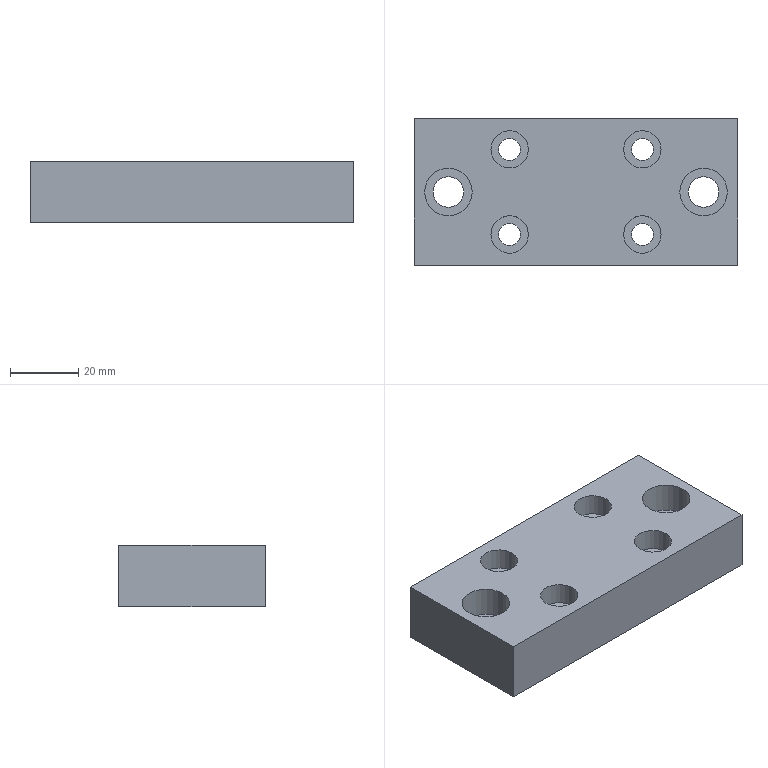Part | STEP file | lll_id474_x_t | 1 solid | 24 faces | box 95 x 43 x 18 mm | volume 65617 mm3 | plane 12 | cylinder 12 | commonest cylinder face diameters 6.5 x4 11 x4 9 x2 14 x2
STEP:
#1=CARTESIAN_POINT('',(47.5,65.,137.5));
#2=VERTEX_POINT('',#1);
#3=CARTESIAN_POINT('',(-47.5,65.,137.5));
#4=VERTEX_POINT('',#3);
#5=CARTESIAN_POINT('',(0.,65.,137.5));
#6=DIRECTION('',(-1.,0.,0.));
#7=VECTOR('',#6,1.);
#8=LINE('',#5,#7);
#9=EDGE_CURVE('',#2,#4,#8,.T.);
#10=ORIENTED_EDGE('',*,*,#9,.F.);
#11=CARTESIAN_POINT('',(47.5,65.,155.5));
#12=VERTEX_POINT('',#11);
#13=CARTESIAN_POINT('',(47.5,65.,155.5));
#14=DIRECTION('',(0.,0.,-1.));
#15=VECTOR('',#14,1.);
#16=LINE('',#13,#15);
#17=EDGE_CURVE('',#12,#2,#16,.T.);
#18=ORIENTED_EDGE('',*,*,#17,.F.);
#19=CARTESIAN_POINT('',(-47.5,65.,155.5));
#20=VERTEX_POINT('',#19);
#21=CARTESIAN_POINT('',(0.,65.,155.5));
#22=DIRECTION('',(-1.,0.,0.));
#23=VECTOR('',#22,1.);
#24=LINE('',#21,#23);
#25=EDGE_CURVE('',#12,#20,#24,.T.);
#26=ORIENTED_EDGE('',*,*,#25,.T.);
#27=CARTESIAN_POINT('',(-47.5,65.,155.5));
#28=DIRECTION('',(0.,0.,-1.));
#29=VECTOR('',#28,1.);
#30=LINE('',#27,#29);
#31=EDGE_CURVE('',#20,#4,#30,.T.);
#32=ORIENTED_EDGE('',*,*,#31,.T.);
#33=EDGE_LOOP('',(#10,#18,#26,#32));
#34=FACE_OUTER_BOUND('',#33,.T.);
#35=CARTESIAN_POINT('',(0.,65.,155.5));
#36=DIRECTION('',(0.,-1.,0.));
#37=DIRECTION('',(0.,0.,-1.));
#38=AXIS2_PLACEMENT_3D('',#35,#36,#37);
#39=PLANE('',#38);
#40=ADVANCED_FACE('',(#34),#39,.T.);
#41=CARTESIAN_POINT('',(47.5,108.,137.5));
#42=VERTEX_POINT('',#41);
#43=CARTESIAN_POINT('',(47.5,140.161,137.5));
#44=DIRECTION('',(0.,-1.,0.));
#45=VECTOR('',#44,1.);
#46=LINE('',#43,#45);
#47=EDGE_CURVE('',#42,#2,#46,.T.);
#48=ORIENTED_EDGE('',*,*,#47,.F.);
#49=CARTESIAN_POINT('',(47.5,108.,155.5));
#50=VERTEX_POINT('',#49);
#51=CARTESIAN_POINT('',(47.5,108.,155.5));
#52=DIRECTION('',(0.,0.,-1.));
#53=VECTOR('',#52,1.);
#54=LINE('',#51,#53);
#55=EDGE_CURVE('',#50,#42,#54,.T.);
#56=ORIENTED_EDGE('',*,*,#55,.F.);
#57=CARTESIAN_POINT('',(47.5,140.161,155.5));
#58=DIRECTION('',(0.,-1.,0.));
#59=VECTOR('',#58,1.);
#60=LINE('',#57,#59);
#61=EDGE_CURVE('',#50,#12,#60,.T.);
#62=ORIENTED_EDGE('',*,*,#61,.T.);
#63=ORIENTED_EDGE('',*,*,#17,.T.);
#64=EDGE_LOOP('',(#48,#56,#62,#63));
#65=FACE_OUTER_BOUND('',#64,.T.);
#66=CARTESIAN_POINT('',(47.5,140.161,155.5));
#67=DIRECTION('',(1.,0.,0.));
#68=DIRECTION('',(0.,0.,-1.));
#69=AXIS2_PLACEMENT_3D('',#66,#67,#68);
#70=PLANE('',#69);
#71=ADVANCED_FACE('',(#65),#70,.T.);
#72=CARTESIAN_POINT('',(-47.5,108.,137.5));
#73=VERTEX_POINT('',#72);
#74=CARTESIAN_POINT('',(0.,108.,137.5));
#75=DIRECTION('',(-1.,0.,0.));
#76=VECTOR('',#75,1.);
#77=LINE('',#74,#76);
#78=EDGE_CURVE('',#42,#73,#77,.T.);
#79=ORIENTED_EDGE('',*,*,#78,.T.);
#80=CARTESIAN_POINT('',(-47.5,108.,155.5));
#81=VERTEX_POINT('',#80);
#82=CARTESIAN_POINT('',(-47.5,108.,155.5));
#83=DIRECTION('',(0.,0.,-1.));
#84=VECTOR('',#83,1.);
#85=LINE('',#82,#84);
#86=EDGE_CURVE('',#81,#73,#85,.T.);
#87=ORIENTED_EDGE('',*,*,#86,.F.);
#88=CARTESIAN_POINT('',(0.,108.,155.5));
#89=DIRECTION('',(-1.,0.,0.));
#90=VECTOR('',#89,1.);
#91=LINE('',#88,#90);
#92=EDGE_CURVE('',#50,#81,#91,.T.);
#93=ORIENTED_EDGE('',*,*,#92,.F.);
#94=ORIENTED_EDGE('',*,*,#55,.T.);
#95=EDGE_LOOP('',(#79,#87,#93,#94));
#96=FACE_OUTER_BOUND('',#95,.T.);
#97=CARTESIAN_POINT('',(0.,108.,155.5));
#98=DIRECTION('',(0.,-1.,0.));
#99=DIRECTION('',(0.,0.,-1.));
#100=AXIS2_PLACEMENT_3D('',#97,#98,#99);
#101=PLANE('',#100);
#102=ADVANCED_FACE('',(#96),#101,.F.);
#103=CARTESIAN_POINT('',(-47.5,0.,137.5));
#104=DIRECTION('',(0.,-1.,0.));
#105=VECTOR('',#104,1.);
#106=LINE('',#103,#105);
#107=EDGE_CURVE('',#73,#4,#106,.T.);
#108=ORIENTED_EDGE('',*,*,#107,.T.);
#109=ORIENTED_EDGE('',*,*,#31,.F.);
#110=CARTESIAN_POINT('',(-47.5,0.,155.5));
#111=DIRECTION('',(0.,-1.,0.));
#112=VECTOR('',#111,1.);
#113=LINE('',#110,#112);
#114=EDGE_CURVE('',#81,#20,#113,.T.);
#115=ORIENTED_EDGE('',*,*,#114,.F.);
#116=ORIENTED_EDGE('',*,*,#86,.T.);
#117=EDGE_LOOP('',(#108,#109,#115,#116));
#118=FACE_OUTER_BOUND('',#117,.T.);
#119=CARTESIAN_POINT('',(-47.5,0.,155.5));
#120=DIRECTION('',(1.,0.,0.));
#121=DIRECTION('',(0.,0.,-1.));
#122=AXIS2_PLACEMENT_3D('',#119,#120,#121);
#123=PLANE('',#122);
#124=ADVANCED_FACE('',(#118),#123,.F.);
#125=CARTESIAN_POINT('',(25.,99.,155.5));
#126=VERTEX_POINT('',#125);
#127=CARTESIAN_POINT('',(19.5,99.,155.5));
#128=DIRECTION('',(0.,0.,-1.));
#129=DIRECTION('',(1.,0.,0.));
#130=AXIS2_PLACEMENT_3D('',#127,#128,#129);
#131=CIRCLE('',#130,5.5);
#132=EDGE_CURVE('',#126,#126,#131,.T.);
#133=ORIENTED_EDGE('',*,*,#132,.T.);
#134=EDGE_LOOP('',(#133));
#135=FACE_BOUND('',#134,.T.);
#136=CARTESIAN_POINT('',(-25.,99.,155.5));
#137=VERTEX_POINT('',#136);
#138=CARTESIAN_POINT('',(-19.5,99.,155.5));
#139=DIRECTION('',(0.,0.,1.));
#140=DIRECTION('',(-1.,0.,0.));
#141=AXIS2_PLACEMENT_3D('',#138,#139,#140);
#142=CIRCLE('',#141,5.5);
#143=EDGE_CURVE('',#137,#137,#142,.T.);
#144=ORIENTED_EDGE('',*,*,#143,.F.);
#145=EDGE_LOOP('',(#144));
#146=FACE_BOUND('',#145,.T.);
#147=CARTESIAN_POINT('',(25.,74.,155.5));
#148=VERTEX_POINT('',#147);
#149=CARTESIAN_POINT('',(19.5,74.,155.5));
#150=DIRECTION('',(0.,0.,1.));
#151=DIRECTION('',(1.,0.,0.));
#152=AXIS2_PLACEMENT_3D('',#149,#150,#151);
#153=CIRCLE('',#152,5.5);
#154=EDGE_CURVE('',#148,#148,#153,.T.);
#155=ORIENTED_EDGE('',*,*,#154,.F.);
#156=EDGE_LOOP('',(#155));
#157=FACE_BOUND('',#156,.T.);
#158=CARTESIAN_POINT('',(-25.,74.,155.5));
#159=VERTEX_POINT('',#158);
#160=CARTESIAN_POINT('',(-19.5,74.,155.5));
#161=DIRECTION('',(0.,0.,-1.));
#162=DIRECTION('',(-1.,0.,0.));
#163=AXIS2_PLACEMENT_3D('',#160,#161,#162);
#164=CIRCLE('',#163,5.5);
#165=EDGE_CURVE('',#159,#159,#164,.T.);
#166=ORIENTED_EDGE('',*,*,#165,.T.);
#167=EDGE_LOOP('',(#166));
#168=FACE_BOUND('',#167,.T.);
#169=CARTESIAN_POINT('',(-30.5,86.5,155.5));
#170=VERTEX_POINT('',#169);
#171=CARTESIAN_POINT('',(-37.5,86.5,155.5));
#172=DIRECTION('',(0.,0.,1.));
#173=DIRECTION('',(1.,0.,0.));
#174=AXIS2_PLACEMENT_3D('',#171,#172,#173);
#175=CIRCLE('',#174,7.);
#176=EDGE_CURVE('',#170,#170,#175,.T.);
#177=ORIENTED_EDGE('',*,*,#176,.F.);
#178=EDGE_LOOP('',(#177));
#179=FACE_BOUND('',#178,.T.);
#180=CARTESIAN_POINT('',(30.5,86.5,155.5));
#181=VERTEX_POINT('',#180);
#182=CARTESIAN_POINT('',(37.5,86.5,155.5));
#183=DIRECTION('',(0.,0.,-1.));
#184=DIRECTION('',(-1.,0.,0.));
#185=AXIS2_PLACEMENT_3D('',#182,#183,#184);
#186=CIRCLE('',#185,7.);
#187=EDGE_CURVE('',#181,#181,#186,.T.);
#188=ORIENTED_EDGE('',*,*,#187,.T.);
#189=EDGE_LOOP('',(#188));
#190=FACE_BOUND('',#189,.T.);
#191=ORIENTED_EDGE('',*,*,#25,.F.);
#192=ORIENTED_EDGE('',*,*,#61,.F.);
#193=ORIENTED_EDGE('',*,*,#92,.T.);
#194=ORIENTED_EDGE('',*,*,#114,.T.);
#195=EDGE_LOOP('',(#191,#192,#193,#194));
#196=FACE_BOUND('',#195,.T.);
#197=CARTESIAN_POINT('',(0.,0.,155.5));
#198=DIRECTION('',(0.,0.,1.));
#199=DIRECTION('',(1.,0.,0.));
#200=AXIS2_PLACEMENT_3D('',#197,#198,#199);
#201=PLANE('',#200);
#202=ADVANCED_FACE('',(#135,#146,#157,#168,#179,#190,#196),#201,.T.);
#203=CARTESIAN_POINT('',(22.75,99.,137.5));
#204=VERTEX_POINT('',#203);
#205=CARTESIAN_POINT('',(19.5,99.,137.5));
#206=DIRECTION('',(0.,0.,1.));
#207=DIRECTION('',(1.,0.,0.));
#208=AXIS2_PLACEMENT_3D('',#205,#206,#207);
#209=CIRCLE('',#208,3.25);
#210=EDGE_CURVE('',#204,#204,#209,.T.);
#211=ORIENTED_EDGE('',*,*,#210,.T.);
#212=EDGE_LOOP('',(#211));
#213=FACE_BOUND('',#212,.T.);
#214=CARTESIAN_POINT('',(-16.25,99.,137.5));
#215=VERTEX_POINT('',#214);
#216=CARTESIAN_POINT('',(-19.5,99.,137.5));
#217=DIRECTION('',(0.,0.,1.));
#218=DIRECTION('',(1.,0.,0.));
#219=AXIS2_PLACEMENT_3D('',#216,#217,#218);
#220=CIRCLE('',#219,3.25);
#221=EDGE_CURVE('',#215,#215,#220,.T.);
#222=ORIENTED_EDGE('',*,*,#221,.T.);
#223=EDGE_LOOP('',(#222));
#224=FACE_BOUND('',#223,.T.);
#225=CARTESIAN_POINT('',(22.75,74.,137.5));
#226=VERTEX_POINT('',#225);
#227=CARTESIAN_POINT('',(19.5,74.,137.5));
#228=DIRECTION('',(0.,0.,1.));
#229=DIRECTION('',(1.,0.,0.));
#230=AXIS2_PLACEMENT_3D('',#227,#228,#229);
#231=CIRCLE('',#230,3.25);
#232=EDGE_CURVE('',#226,#226,#231,.T.);
#233=ORIENTED_EDGE('',*,*,#232,.T.);
#234=EDGE_LOOP('',(#233));
#235=FACE_BOUND('',#234,.T.);
#236=CARTESIAN_POINT('',(-16.25,74.,137.5));
#237=VERTEX_POINT('',#236);
#238=CARTESIAN_POINT('',(-19.5,74.,137.5));
#239=DIRECTION('',(0.,0.,1.));
#240=DIRECTION('',(1.,0.,0.));
#241=AXIS2_PLACEMENT_3D('',#238,#239,#240);
#242=CIRCLE('',#241,3.25);
#243=EDGE_CURVE('',#237,#237,#242,.T.);
#244=ORIENTED_EDGE('',*,*,#243,.T.);
#245=EDGE_LOOP('',(#244));
#246=FACE_BOUND('',#245,.T.);
#247=CARTESIAN_POINT('',(-33.,86.5,137.5));
#248=VERTEX_POINT('',#247);
#249=CARTESIAN_POINT('',(-37.5,86.5,137.5));
#250=DIRECTION('',(0.,0.,1.));
#251=DIRECTION('',(1.,0.,0.));
#252=AXIS2_PLACEMENT_3D('',#249,#250,#251);
#253=CIRCLE('',#252,4.5);
#254=EDGE_CURVE('',#248,#248,#253,.T.);
#255=ORIENTED_EDGE('',*,*,#254,.T.);
#256=EDGE_LOOP('',(#255));
#257=FACE_BOUND('',#256,.T.);
#258=CARTESIAN_POINT('',(42.,86.5,137.5));
#259=VERTEX_POINT('',#258);
#260=CARTESIAN_POINT('',(37.5,86.5,137.5));
#261=DIRECTION('',(0.,0.,1.));
#262=DIRECTION('',(1.,0.,0.));
#263=AXIS2_PLACEMENT_3D('',#260,#261,#262);
#264=CIRCLE('',#263,4.5);
#265=EDGE_CURVE('',#259,#259,#264,.T.);
#266=ORIENTED_EDGE('',*,*,#265,.T.);
#267=EDGE_LOOP('',(#266));
#268=FACE_BOUND('',#267,.T.);
#269=ORIENTED_EDGE('',*,*,#9,.T.);
#270=ORIENTED_EDGE('',*,*,#107,.F.);
#271=ORIENTED_EDGE('',*,*,#78,.F.);
#272=ORIENTED_EDGE('',*,*,#47,.T.);
#273=EDGE_LOOP('',(#269,#270,#271,#272));
#274=FACE_BOUND('',#273,.T.);
#275=CARTESIAN_POINT('',(0.,0.,137.5));
#276=DIRECTION('',(0.,0.,1.));
#277=DIRECTION('',(1.,0.,0.));
#278=AXIS2_PLACEMENT_3D('',#275,#276,#277);
#279=PLANE('',#278);
#280=ADVANCED_FACE('',(#213,#224,#235,#246,#257,#268,#274),#279,.F.);
#281=CARTESIAN_POINT('',(33.,86.5,146.5));
#282=VERTEX_POINT('',#281);
#283=CARTESIAN_POINT('',(37.5,86.5,146.5));
#284=DIRECTION('',(0.,0.,-1.));
#285=DIRECTION('',(-1.,0.,0.));
#286=AXIS2_PLACEMENT_3D('',#283,#284,#285);
#287=CIRCLE('',#286,4.5);
#288=EDGE_CURVE('',#282,#282,#287,.T.);
#289=ORIENTED_EDGE('',*,*,#288,.F.);
#290=EDGE_LOOP('',(#289));
#291=FACE_BOUND('',#290,.T.);
#292=ORIENTED_EDGE('',*,*,#265,.F.);
#293=EDGE_LOOP('',(#292));
#294=FACE_BOUND('',#293,.T.);
#295=CARTESIAN_POINT('',(37.5,86.5,105.5));
#296=DIRECTION('',(0.,0.,-1.));
#297=DIRECTION('',(-1.,0.,0.));
#298=AXIS2_PLACEMENT_3D('',#295,#296,#297);
#299=CYLINDRICAL_SURFACE('',#298,4.5);
#300=ADVANCED_FACE('',(#291,#294),#299,.F.);
#301=ORIENTED_EDGE('',*,*,#288,.T.);
#302=EDGE_LOOP('',(#301));
#303=FACE_BOUND('',#302,.T.);
#304=CARTESIAN_POINT('',(30.5,86.5,146.5));
#305=VERTEX_POINT('',#304);
#306=CARTESIAN_POINT('',(37.5,86.5,146.5));
#307=DIRECTION('',(0.,0.,-1.));
#308=DIRECTION('',(-1.,0.,0.));
#309=AXIS2_PLACEMENT_3D('',#306,#307,#308);
#310=CIRCLE('',#309,7.);
#311=EDGE_CURVE('',#305,#305,#310,.T.);
#312=ORIENTED_EDGE('',*,*,#311,.F.);
#313=EDGE_LOOP('',(#312));
#314=FACE_BOUND('',#313,.T.);
#315=CARTESIAN_POINT('',(37.5,86.5,146.5));
#316=DIRECTION('',(0.,0.,-1.));
#317=DIRECTION('',(-1.,0.,0.));
#318=AXIS2_PLACEMENT_3D('',#315,#316,#317);
#319=PLANE('',#318);
#320=ADVANCED_FACE('',(#303,#314),#319,.F.);
#321=ORIENTED_EDGE('',*,*,#311,.T.);
#322=EDGE_LOOP('',(#321));
#323=FACE_BOUND('',#322,.T.);
#324=ORIENTED_EDGE('',*,*,#187,.F.);
#325=EDGE_LOOP('',(#324));
#326=FACE_BOUND('',#325,.T.);
#327=CARTESIAN_POINT('',(37.5,86.5,155.5));
#328=DIRECTION('',(0.,0.,-1.));
#329=DIRECTION('',(-1.,0.,0.));
#330=AXIS2_PLACEMENT_3D('',#327,#328,#329);
#331=CYLINDRICAL_SURFACE('',#330,7.);
#332=ADVANCED_FACE('',(#323,#326),#331,.F.);
#333=CARTESIAN_POINT('',(-33.,86.5,146.5));
#334=VERTEX_POINT('',#333);
#335=CARTESIAN_POINT('',(-37.5,86.5,146.5));
#336=DIRECTION('',(0.,0.,1.));
#337=DIRECTION('',(1.,0.,0.));
#338=AXIS2_PLACEMENT_3D('',#335,#336,#337);
#339=CIRCLE('',#338,4.5);
#340=EDGE_CURVE('',#334,#334,#339,.T.);
#341=ORIENTED_EDGE('',*,*,#340,.T.);
#342=EDGE_LOOP('',(#341));
#343=FACE_BOUND('',#342,.T.);
#344=ORIENTED_EDGE('',*,*,#254,.F.);
#345=EDGE_LOOP('',(#344));
#346=FACE_BOUND('',#345,.T.);
#347=CARTESIAN_POINT('',(-37.5,86.5,105.5));
#348=DIRECTION('',(0.,0.,-1.));
#349=DIRECTION('',(1.,0.,0.));
#350=AXIS2_PLACEMENT_3D('',#347,#348,#349);
#351=CYLINDRICAL_SURFACE('',#350,4.5);
#352=ADVANCED_FACE('',(#343,#346),#351,.F.);
#353=ORIENTED_EDGE('',*,*,#340,.F.);
#354=EDGE_LOOP('',(#353));
#355=FACE_BOUND('',#354,.T.);
#356=CARTESIAN_POINT('',(-30.5,86.5,146.5));
#357=VERTEX_POINT('',#356);
#358=CARTESIAN_POINT('',(-37.5,86.5,146.5));
#359=DIRECTION('',(0.,0.,1.));
#360=DIRECTION('',(1.,0.,0.));
#361=AXIS2_PLACEMENT_3D('',#358,#359,#360);
#362=CIRCLE('',#361,7.);
#363=EDGE_CURVE('',#357,#357,#362,.T.);
#364=ORIENTED_EDGE('',*,*,#363,.T.);
#365=EDGE_LOOP('',(#364));
#366=FACE_BOUND('',#365,.T.);
#367=CARTESIAN_POINT('',(-37.5,86.5,146.5));
#368=DIRECTION('',(0.,0.,-1.));
#369=DIRECTION('',(1.,0.,0.));
#370=AXIS2_PLACEMENT_3D('',#367,#368,#369);
#371=PLANE('',#370);
#372=ADVANCED_FACE('',(#355,#366),#371,.F.);
#373=ORIENTED_EDGE('',*,*,#363,.F.);
#374=EDGE_LOOP('',(#373));
#375=FACE_BOUND('',#374,.T.);
#376=ORIENTED_EDGE('',*,*,#176,.T.);
#377=EDGE_LOOP('',(#376));
#378=FACE_BOUND('',#377,.T.);
#379=CARTESIAN_POINT('',(-37.5,86.5,155.5));
#380=DIRECTION('',(0.,0.,-1.));
#381=DIRECTION('',(1.,0.,0.));
#382=AXIS2_PLACEMENT_3D('',#379,#380,#381);
#383=CYLINDRICAL_SURFACE('',#382,7.);
#384=ADVANCED_FACE('',(#375,#378),#383,.F.);
#385=CARTESIAN_POINT('',(-22.75,74.,149.));
#386=VERTEX_POINT('',#385);
#387=CARTESIAN_POINT('',(-19.5,74.,149.));
#388=DIRECTION('',(0.,0.,-1.));
#389=DIRECTION('',(-1.,0.,0.));
#390=AXIS2_PLACEMENT_3D('',#387,#388,#389);
#391=CIRCLE('',#390,3.25);
#392=EDGE_CURVE('',#386,#386,#391,.T.);
#393=ORIENTED_EDGE('',*,*,#392,.F.);
#394=EDGE_LOOP('',(#393));
#395=FACE_BOUND('',#394,.T.);
#396=ORIENTED_EDGE('',*,*,#243,.F.);
#397=EDGE_LOOP('',(#396));
#398=FACE_BOUND('',#397,.T.);
#399=CARTESIAN_POINT('',(-19.5,74.,-144.5));
#400=DIRECTION('',(0.,0.,-1.));
#401=DIRECTION('',(-1.,0.,0.));
#402=AXIS2_PLACEMENT_3D('',#399,#400,#401);
#403=CYLINDRICAL_SURFACE('',#402,3.25);
#404=ADVANCED_FACE('',(#395,#398),#403,.F.);
#405=ORIENTED_EDGE('',*,*,#392,.T.);
#406=EDGE_LOOP('',(#405));
#407=FACE_BOUND('',#406,.T.);
#408=CARTESIAN_POINT('',(-25.,74.,149.));
#409=VERTEX_POINT('',#408);
#410=CARTESIAN_POINT('',(-19.5,74.,149.));
#411=DIRECTION('',(0.,0.,-1.));
#412=DIRECTION('',(-1.,0.,0.));
#413=AXIS2_PLACEMENT_3D('',#410,#411,#412);
#414=CIRCLE('',#413,5.5);
#415=EDGE_CURVE('',#409,#409,#414,.T.);
#416=ORIENTED_EDGE('',*,*,#415,.F.);
#417=EDGE_LOOP('',(#416));
#418=FACE_BOUND('',#417,.T.);
#419=CARTESIAN_POINT('',(-19.5,74.,149.));
#420=DIRECTION('',(0.,0.,-1.));
#421=DIRECTION('',(-1.,0.,0.));
#422=AXIS2_PLACEMENT_3D('',#419,#420,#421);
#423=PLANE('',#422);
#424=ADVANCED_FACE('',(#407,#418),#423,.F.);
#425=ORIENTED_EDGE('',*,*,#415,.T.);
#426=EDGE_LOOP('',(#425));
#427=FACE_BOUND('',#426,.T.);
#428=ORIENTED_EDGE('',*,*,#165,.F.);
#429=EDGE_LOOP('',(#428));
#430=FACE_BOUND('',#429,.T.);
#431=CARTESIAN_POINT('',(-19.5,74.,155.5));
#432=DIRECTION('',(0.,0.,-1.));
#433=DIRECTION('',(-1.,0.,0.));
#434=AXIS2_PLACEMENT_3D('',#431,#432,#433);
#435=CYLINDRICAL_SURFACE('',#434,5.5);
#436=ADVANCED_FACE('',(#427,#430),#435,.F.);
#437=CARTESIAN_POINT('',(22.75,74.,149.));
#438=VERTEX_POINT('',#437);
#439=CARTESIAN_POINT('',(19.5,74.,149.));
#440=DIRECTION('',(0.,0.,1.));
#441=DIRECTION('',(1.,0.,0.));
#442=AXIS2_PLACEMENT_3D('',#439,#440,#441);
#443=CIRCLE('',#442,3.25);
#444=EDGE_CURVE('',#438,#438,#443,.T.);
#445=ORIENTED_EDGE('',*,*,#444,.T.);
#446=EDGE_LOOP('',(#445));
#447=FACE_BOUND('',#446,.T.);
#448=ORIENTED_EDGE('',*,*,#232,.F.);
#449=EDGE_LOOP('',(#448));
#450=FACE_BOUND('',#449,.T.);
#451=CARTESIAN_POINT('',(19.5,74.,-144.5));
#452=DIRECTION('',(0.,0.,-1.));
#453=DIRECTION('',(1.,0.,0.));
#454=AXIS2_PLACEMENT_3D('',#451,#452,#453);
#455=CYLINDRICAL_SURFACE('',#454,3.25);
#456=ADVANCED_FACE('',(#447,#450),#455,.F.);
#457=ORIENTED_EDGE('',*,*,#444,.F.);
#458=EDGE_LOOP('',(#457));
#459=FACE_BOUND('',#458,.T.);
#460=CARTESIAN_POINT('',(25.,74.,149.));
#461=VERTEX_POINT('',#460);
#462=CARTESIAN_POINT('',(19.5,74.,149.));
#463=DIRECTION('',(0.,0.,1.));
#464=DIRECTION('',(1.,0.,0.));
#465=AXIS2_PLACEMENT_3D('',#462,#463,#464);
#466=CIRCLE('',#465,5.5);
#467=EDGE_CURVE('',#461,#461,#466,.T.);
#468=ORIENTED_EDGE('',*,*,#467,.T.);
#469=EDGE_LOOP('',(#468));
#470=FACE_BOUND('',#469,.T.);
#471=CARTESIAN_POINT('',(19.5,74.,149.));
#472=DIRECTION('',(0.,0.,-1.));
#473=DIRECTION('',(1.,0.,0.));
#474=AXIS2_PLACEMENT_3D('',#471,#472,#473);
#475=PLANE('',#474);
#476=ADVANCED_FACE('',(#459,#470),#475,.F.);
#477=ORIENTED_EDGE('',*,*,#467,.F.);
#478=EDGE_LOOP('',(#477));
#479=FACE_BOUND('',#478,.T.);
#480=ORIENTED_EDGE('',*,*,#154,.T.);
#481=EDGE_LOOP('',(#480));
#482=FACE_BOUND('',#481,.T.);
#483=CARTESIAN_POINT('',(19.5,74.,155.5));
#484=DIRECTION('',(0.,0.,-1.));
#485=DIRECTION('',(1.,0.,0.));
#486=AXIS2_PLACEMENT_3D('',#483,#484,#485);
#487=CYLINDRICAL_SURFACE('',#486,5.5);
#488=ADVANCED_FACE('',(#479,#482),#487,.F.);
#489=CARTESIAN_POINT('',(-22.75,99.,149.));
#490=VERTEX_POINT('',#489);
#491=CARTESIAN_POINT('',(-19.5,99.,149.));
#492=DIRECTION('',(0.,0.,1.));
#493=DIRECTION('',(-1.,0.,0.));
#494=AXIS2_PLACEMENT_3D('',#491,#492,#493);
#495=CIRCLE('',#494,3.25);
#496=EDGE_CURVE('',#490,#490,#495,.T.);
#497=ORIENTED_EDGE('',*,*,#496,.T.);
#498=EDGE_LOOP('',(#497));
#499=FACE_BOUND('',#498,.T.);
#500=ORIENTED_EDGE('',*,*,#221,.F.);
#501=EDGE_LOOP('',(#500));
#502=FACE_BOUND('',#501,.T.);
#503=CARTESIAN_POINT('',(-19.5,99.,-144.5));
#504=DIRECTION('',(0.,0.,-1.));
#505=DIRECTION('',(-1.,0.,0.));
#506=AXIS2_PLACEMENT_3D('',#503,#504,#505);
#507=CYLINDRICAL_SURFACE('',#506,3.25);
#508=ADVANCED_FACE('',(#499,#502),#507,.F.);
#509=ORIENTED_EDGE('',*,*,#496,.F.);
#510=EDGE_LOOP('',(#509));
#511=FACE_BOUND('',#510,.T.);
#512=CARTESIAN_POINT('',(-25.,99.,149.));
#513=VERTEX_POINT('',#512);
#514=CARTESIAN_POINT('',(-19.5,99.,149.));
#515=DIRECTION('',(0.,0.,1.));
#516=DIRECTION('',(-1.,0.,0.));
#517=AXIS2_PLACEMENT_3D('',#514,#515,#516);
#518=CIRCLE('',#517,5.5);
#519=EDGE_CURVE('',#513,#513,#518,.T.);
#520=ORIENTED_EDGE('',*,*,#519,.T.);
#521=EDGE_LOOP('',(#520));
#522=FACE_BOUND('',#521,.T.);
#523=CARTESIAN_POINT('',(-19.5,99.,149.));
#524=DIRECTION('',(0.,0.,-1.));
#525=DIRECTION('',(-1.,0.,0.));
#526=AXIS2_PLACEMENT_3D('',#523,#524,#525);
#527=PLANE('',#526);
#528=ADVANCED_FACE('',(#511,#522),#527,.F.);
#529=ORIENTED_EDGE('',*,*,#519,.F.);
#530=EDGE_LOOP('',(#529));
#531=FACE_BOUND('',#530,.T.);
#532=ORIENTED_EDGE('',*,*,#143,.T.);
#533=EDGE_LOOP('',(#532));
#534=FACE_BOUND('',#533,.T.);
#535=CARTESIAN_POINT('',(-19.5,99.,155.5));
#536=DIRECTION('',(0.,0.,-1.));
#537=DIRECTION('',(-1.,0.,0.));
#538=AXIS2_PLACEMENT_3D('',#535,#536,#537);
#539=CYLINDRICAL_SURFACE('',#538,5.5);
#540=ADVANCED_FACE('',(#531,#534),#539,.F.);
#541=CARTESIAN_POINT('',(22.75,99.,149.));
#542=VERTEX_POINT('',#541);
#543=CARTESIAN_POINT('',(19.5,99.,149.));
#544=DIRECTION('',(0.,0.,-1.));
#545=DIRECTION('',(1.,0.,0.));
#546=AXIS2_PLACEMENT_3D('',#543,#544,#545);
#547=CIRCLE('',#546,3.25);
#548=EDGE_CURVE('',#542,#542,#547,.T.);
#549=ORIENTED_EDGE('',*,*,#548,.F.);
#550=EDGE_LOOP('',(#549));
#551=FACE_BOUND('',#550,.T.);
#552=ORIENTED_EDGE('',*,*,#210,.F.);
#553=EDGE_LOOP('',(#552));
#554=FACE_BOUND('',#553,.T.);
#555=CARTESIAN_POINT('',(19.5,99.,-144.5));
#556=DIRECTION('',(0.,0.,-1.));
#557=DIRECTION('',(1.,0.,0.));
#558=AXIS2_PLACEMENT_3D('',#555,#556,#557);
#559=CYLINDRICAL_SURFACE('',#558,3.25);
#560=ADVANCED_FACE('',(#551,#554),#559,.F.);
#561=ORIENTED_EDGE('',*,*,#548,.T.);
#562=EDGE_LOOP('',(#561));
#563=FACE_BOUND('',#562,.T.);
#564=CARTESIAN_POINT('',(25.,99.,149.));
#565=VERTEX_POINT('',#564);
#566=CARTESIAN_POINT('',(19.5,99.,149.));
#567=DIRECTION('',(0.,0.,-1.));
#568=DIRECTION('',(1.,0.,0.));
#569=AXIS2_PLACEMENT_3D('',#566,#567,#568);
#570=CIRCLE('',#569,5.5);
#571=EDGE_CURVE('',#565,#565,#570,.T.);
#572=ORIENTED_EDGE('',*,*,#571,.F.);
#573=EDGE_LOOP('',(#572));
#574=FACE_BOUND('',#573,.T.);
#575=CARTESIAN_POINT('',(19.5,99.,149.));
#576=DIRECTION('',(0.,0.,-1.));
#577=DIRECTION('',(1.,0.,0.));
#578=AXIS2_PLACEMENT_3D('',#575,#576,#577);
#579=PLANE('',#578);
#580=ADVANCED_FACE('',(#563,#574),#579,.F.);
#581=ORIENTED_EDGE('',*,*,#571,.T.);
#582=EDGE_LOOP('',(#581));
#583=FACE_BOUND('',#582,.T.);
#584=ORIENTED_EDGE('',*,*,#132,.F.);
#585=EDGE_LOOP('',(#584));
#586=FACE_BOUND('',#585,.T.);
#587=CARTESIAN_POINT('',(19.5,99.,155.5));
#588=DIRECTION('',(0.,0.,-1.));
#589=DIRECTION('',(1.,0.,0.));
#590=AXIS2_PLACEMENT_3D('',#587,#588,#589);
#591=CYLINDRICAL_SURFACE('',#590,5.5);
#592=ADVANCED_FACE('',(#583,#586),#591,.F.);
#593=CLOSED_SHELL('',(#40,#71,#102,#124,#202,#280,#300,#320,#332,#352,#372,#384,#404,#424,#436,#456,#476,#488,#508,#528,#540,#560,#580,#592));
#594=MANIFOLD_SOLID_BREP('',#593);
#595=(LENGTH_UNIT()NAMED_UNIT(*)SI_UNIT(.MILLI.,.METRE.));
#596=UNCERTAINTY_MEASURE_WITH_UNIT(LENGTH_MEASURE(0.00002),#595,'','');
#597=(NAMED_UNIT(*)PLANE_ANGLE_UNIT()SI_UNIT($,.RADIAN.));
#598=PLANE_ANGLE_MEASURE_WITH_UNIT(PLANE_ANGLE_MEASURE(0.01745),#597);
#599=DIMENSIONAL_EXPONENTS(0.,0.,0.,0.,0.,0.,0.);
#600=(CONVERSION_BASED_UNIT('DEGREE',#598)NAMED_UNIT(#599)PLANE_ANGLE_UNIT());
#601=(NAMED_UNIT(*)SI_UNIT($,.STERADIAN.)SOLID_ANGLE_UNIT());
#602=(GEOMETRIC_REPRESENTATION_CONTEXT(3)GLOBAL_UNCERTAINTY_ASSIGNED_CONTEXT((#596))GLOBAL_UNIT_ASSIGNED_CONTEXT((#595,#600,#601))REPRESENTATION_CONTEXT('',''));
#603=ADVANCED_BREP_SHAPE_REPRESENTATION('',(#594),#602);